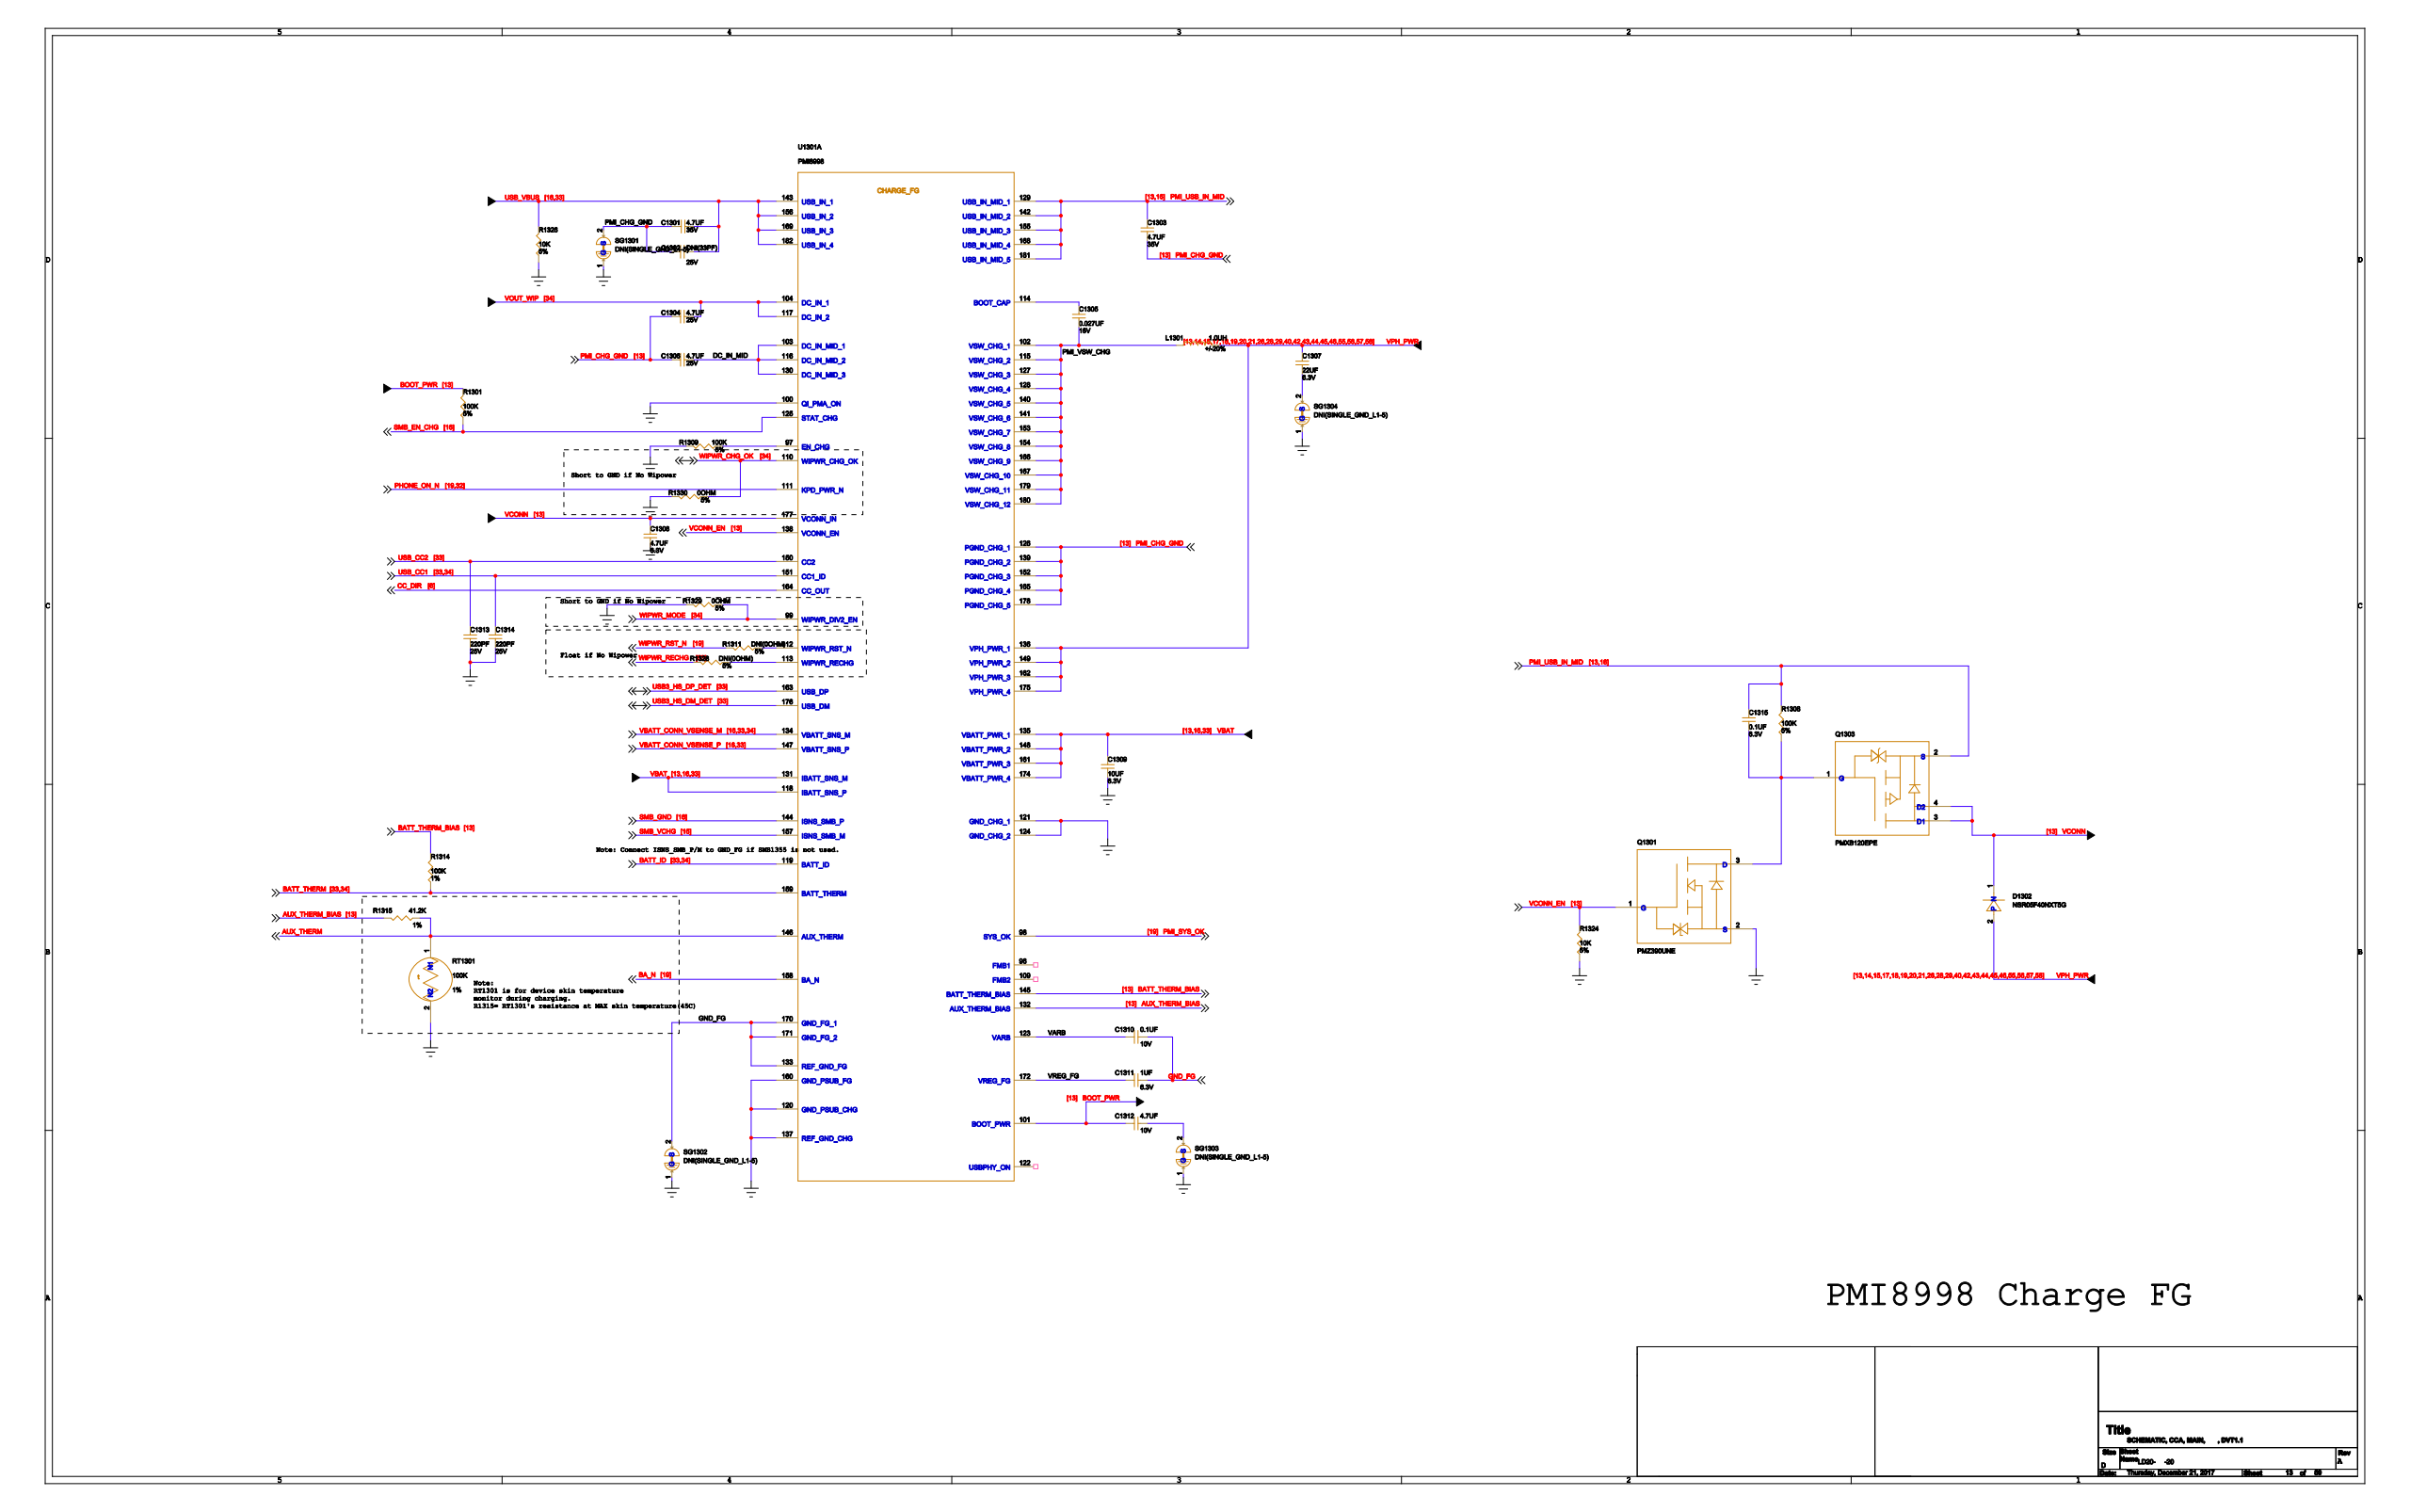Circuit board | Cadence Allegro | 1520 parts | 1149 nets | one sheet of the schematic
Parts on this sheet (reference | value | footprint):
C1301 | 4.7UF | 2P0603R
C1302 | DNI(33PF) | 2P0201R_DNI
C1303 | 4.7UF | 2P0603R
C1304 | 4.7UF | 2P0603R
C1305 | 0.027UF | 2P0402R
C1306 | 4.7UF | 2P0603R
C1307 | 22UF | 2P0603R
C1308 | 4.7UF | 2P0402R
C1309 | 10UF | 2P0402RV1
C1310 | 0.1UF | 2P0201R
C1311 | 1UF | 2P0201R
C1312 | 4.7UF | 2P0402R
C1313 | 220PF | 2P0201R
C1314 | 220PF | 2P0201R
C1315 | 0.1UF | 2P0201R
D1302 | NSR05F40NXT5G | 2PSM39X24NV1
L1301 | 1.0UH | 2PSM106X87RV3
Q1301 | PMZ390UNE | 3PSM43X28N
Q1303 | PMXB120EPE | PMXB360ENEA
R1301 | 100K | 2P0201R
R1308 | 100K | 2P0201R
R1309 | 100K | 2P0201R
R1311 | DNI(0OHM) | 2P0201R_DNI
R1314 | 100K | 2P0201R
R1315 | 41.2K | 2P0201R
R1324 | 10K | 2P0201R
R1326 | 10K | 2P0201R
R1328 | DNI(0OHM) | 2P0201R_DNI
R1329 | 0OHM | 2P0201R
R1330 | 0OHM | 2P0201R
RT1301 | 100K | 2P0201R
SG1301 | DNI(SINGLE_GND_L1-5) | GND_L1-5
SG1302 | DNI(SINGLE_GND_L1-5) | GND_L1-5
SG1303 | DNI(SINGLE_GND_L1-5) | GND_L1-5
SG1304 | DNI(SINGLE_GND_L1-5) | GND_L1-5
U1301 | PMI8998 | 182PGA229X212B157
Nets of these parts (net: part-pin ...):
GND: C1308-2 C1309-2 C1313-2 C1314-2 Q1301-2 R1309-1 R1324-2 R1326-2 R1329-1 R1330-1 RT1301-2 SG1301-1 SG1302-1 SG1303-1 SG1304-1 U1301-15 U1301-18 U1301-43 U1301-59 U1301-100 U1301-120 U1301-121 U1301-124 U1301-137 U1301-160
PMI_CHG_GND: C1301-2 C1302-1 C1303-2 C1304-1 C1306-1 SG1301-2 U1301-126 U1301-139 U1301-152 U1301-165 U1301-178
GND_FG: C1310-2 C1311-2 SG1302-2 U1301-133 U1301-170 U1301-171
N34042291: C1312-2 SG1303-2
N34040602: C1307-2 SG1304-2
SMB_GND: U1301-144
VPH_PWR: C1307-1 D1302-2 L1301-2 U1301-2 U1301-42 U1301-136 U1301-149 U1301-162 U1301-175
VBAT: C1309-1 U1301-118 U1301-131 U1301-135 U1301-148 U1301-161 U1301-174
VBATT_CONN_VSENSE_P: U1301-147
BATT_THERM: R1314-2 U1301-159
BATT_ID: U1301-119
VBATT_CONN_VSENSE_M: U1301-134
AUX_THERM_BIAS: R1315-1 U1301-132
AUX_THERM: R1315-2 RT1301-1 U1301-146
SMB_EN_CHG: R1301-2 U1301-125
USB_VBUS: C1301-1 C1302-2 R1326-1 U1301-143 U1301-156 U1301-169 U1301-182
SMB_VCHG: U1301-157
PMI_USB_IN_MID: C1303-1 C1315-1 Q1303-2 R1308-1 U1301-129 U1301-142 U1301-155 U1301-168 U1301-181
VARB: C1310-1 U1301-123
N34083163: C1315-2 Q1301-3 Q1303-1 R1308-2
VREG_FG: C1311-1 U1301-172
VCONN: C1308-1 D1302-1 Q1303-3 Q1303-4 U1301-177
VOUT_WIP: C1304-2 U1301-104 U1301-117
DC_IN_MID: C1306-2 U1301-103 U1301-116 U1301-130
N34040486: C1305-1 U1301-114
PMI_VSW_CHG: C1305-2 L1301-1 U1301-102 U1301-115 U1301-127 U1301-128 U1301-140 U1301-141 U1301-153 U1301-154 U1301-166 U1301-167 U1301-179 U1301-180
BOOT_PWR: C1312-1 R1301-1 U1301-101
USB_CC2: C1313-1 U1301-150
USB_CC1: C1314-1 U1301-151
WIPWR_MODE: R1329-2 U1301-99
WIPWR_CHG_OK: R1330-2 U1301-110
WIPWR_RECHG: R1328-1
WIPWR_RST_N: R1311-1
N34039466: R1311-2 U1301-112
N49529950: R1328-2 U1301-113
BATT_THERM_BIAS: R1314-1 U1301-145
N34038264: R1309-2 U1301-97
VCONN_EN: Q1301-1 R1324-1 U1301-138
USB3_HS_DM_DET: U1301-176
USB3_HS_DP_DET: U1301-163
PHONE_ON_N: U1301-111
BA_N: U1301-158
CC_DIR: U1301-164
PMI_SYS_OK: U1301-98